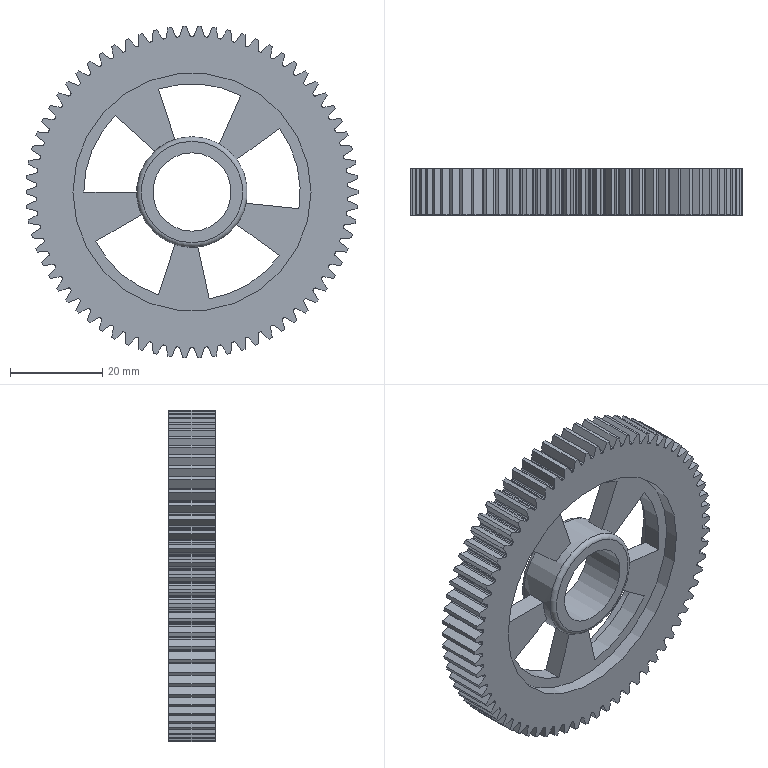Part | NX | features BREP 70, META 70, DATUM_CSYS 4, EXTRUDE 4, SKETCH 3, BLEND 1, CYLINDER 1, FSET 1 | 1 solid | 447 faces | volume 22935 mm3 | spline 350 | cylinder 79 | plane 16 | torus 2 | commonest cylinder face diameters 67.5 x70 46.922 x5 51.634 x2 17 x1 24 x1